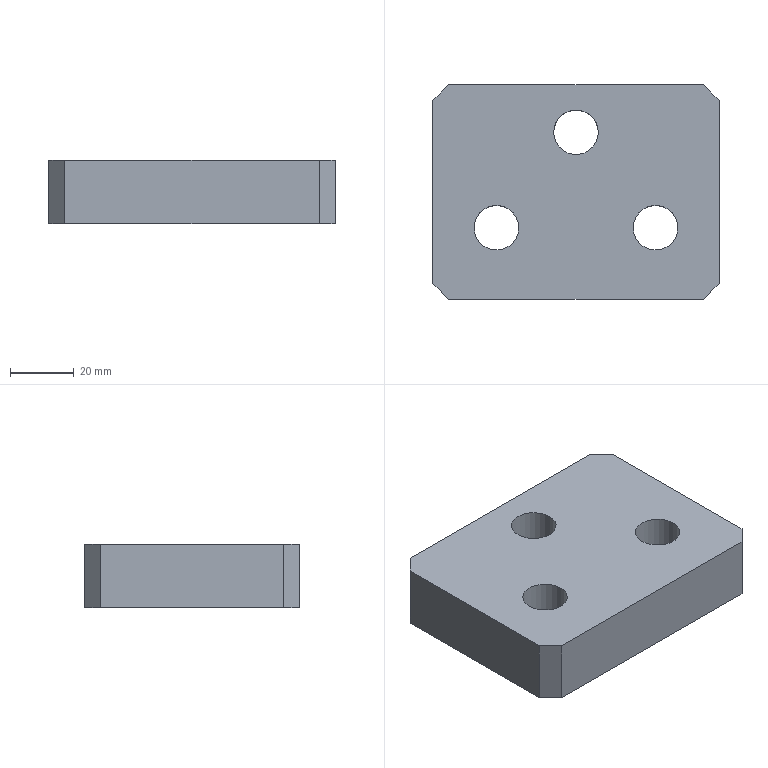Part | STEP file | 1_id1478_x_t | 1 solid | 13 faces | box 90 x 67.5 x 20 mm | volume 111264 mm3 | plane 10 | cylinder 3 | commonest cylinder face diameters 14 x3
STEP:
#1=CARTESIAN_POINT('',(0.,0.,0.));
#2=DIRECTION('',(0.,0.,1.));
#3=DIRECTION('',(1.,0.,0.));
#4=AXIS2_PLACEMENT_3D('',#1,#2,#3);
#5=CARTESIAN_POINT('',(837.95,375.5,-51.89));
#6=VERTEX_POINT('',#5);
#7=CARTESIAN_POINT('',(837.95,375.5,-71.89));
#8=VERTEX_POINT('',#7);
#9=CARTESIAN_POINT('',(837.95,375.5,-51.89));
#10=DIRECTION('',(0.,0.,-1.));
#11=VECTOR('',#10,1.);
#12=LINE('',#9,#11);
#13=CARTESIAN_POINT('',(832.95,375.5,-71.89));
#14=DIRECTION('',(0.,1.,0.));
#15=DIRECTION('',(-1.,0.,0.));
#16=AXIS2_PLACEMENT_3D('',#13,#14,#15);
#17=PLANE('',#16);
#18=CARTESIAN_POINT('',(-5.,20.));
#19=DIRECTION('',(0.,-1.));
#20=VECTOR('',#19,1.);
#21=LINE('',#18,#20);
#22=(GEOMETRIC_REPRESENTATION_CONTEXT(2)PARAMETRIC_REPRESENTATION_CONTEXT()REPRESENTATION_CONTEXT('',''));
#23=DEFINITIONAL_REPRESENTATION('',(#21),#22);
#24=PCURVE('',#17,#23);
#25=CARTESIAN_POINT('',(989.753,223.697,-71.89));
#26=DIRECTION('',(0.7071,0.7071,0.));
#27=DIRECTION('',(-0.7071,0.7071,0.));
#28=AXIS2_PLACEMENT_3D('',#25,#26,#27);
#29=PLANE('',#28);
#30=CARTESIAN_POINT('',(214.682,20.));
#31=DIRECTION('',(0.,-1.));
#32=VECTOR('',#31,1.);
#33=LINE('',#30,#32);
#34=(GEOMETRIC_REPRESENTATION_CONTEXT(2)PARAMETRIC_REPRESENTATION_CONTEXT()REPRESENTATION_CONTEXT('',''));
#35=DEFINITIONAL_REPRESENTATION('',(#33),#34);
#36=PCURVE('',#29,#35);
#37=SURFACE_CURVE('',#12,(#24,#36),.PCURVE_S1.);
#38=EDGE_CURVE('',#6,#8,#37,.T.);
#39=ORIENTED_EDGE('',*,*,#38,.T.);
#40=CARTESIAN_POINT('',(917.95,375.5,-71.89));
#41=VERTEX_POINT('',#40);
#42=CARTESIAN_POINT('',(917.95,375.5,-71.89));
#43=DIRECTION('',(-1.,0.,0.));
#44=VECTOR('',#43,1.);
#45=LINE('',#42,#44);
#46=CARTESIAN_POINT('',(-85.,0.));
#47=DIRECTION('',(1.,0.));
#48=VECTOR('',#47,1.);
#49=LINE('',#46,#48);
#50=(GEOMETRIC_REPRESENTATION_CONTEXT(2)PARAMETRIC_REPRESENTATION_CONTEXT()REPRESENTATION_CONTEXT('',''));
#51=DEFINITIONAL_REPRESENTATION('',(#49),#50);
#52=PCURVE('',#17,#51);
#53=CARTESIAN_POINT('',(739.556,-72.,-71.89));
#54=DIRECTION('',(0.,0.,1.));
#55=DIRECTION('',(1.,0.,0.));
#56=AXIS2_PLACEMENT_3D('',#53,#54,#55);
#57=PLANE('',#56);
#58=CARTESIAN_POINT('',(178.394,447.5));
#59=DIRECTION('',(-1.,0.));
#60=VECTOR('',#59,1.);
#61=LINE('',#58,#60);
#62=(GEOMETRIC_REPRESENTATION_CONTEXT(2)PARAMETRIC_REPRESENTATION_CONTEXT()REPRESENTATION_CONTEXT('',''));
#63=DEFINITIONAL_REPRESENTATION('',(#61),#62);
#64=PCURVE('',#57,#63);
#65=SURFACE_CURVE('',#45,(#52,#64),.PCURVE_S1.);
#66=EDGE_CURVE('',#41,#8,#65,.T.);
#67=ORIENTED_EDGE('',*,*,#66,.F.);
#68=CARTESIAN_POINT('',(917.95,375.5,-51.89));
#69=VERTEX_POINT('',#68);
#70=CARTESIAN_POINT('',(917.95,375.5,-51.89));
#71=DIRECTION('',(0.,0.,-1.));
#72=VECTOR('',#71,1.);
#73=LINE('',#70,#72);
#74=CARTESIAN_POINT('',(-85.,20.));
#75=DIRECTION('',(0.,-1.));
#76=VECTOR('',#75,1.);
#77=LINE('',#74,#76);
#78=(GEOMETRIC_REPRESENTATION_CONTEXT(2)PARAMETRIC_REPRESENTATION_CONTEXT()REPRESENTATION_CONTEXT('',''));
#79=DEFINITIONAL_REPRESENTATION('',(#77),#78);
#80=PCURVE('',#17,#79);
#81=CARTESIAN_POINT('',(577.753,35.303,-71.89));
#82=DIRECTION('',(-0.7071,0.7071,0.));
#83=DIRECTION('',(-0.7071,-0.7071,0.));
#84=AXIS2_PLACEMENT_3D('',#81,#82,#83);
#85=PLANE('',#84);
#86=CARTESIAN_POINT('',(-481.111,20.));
#87=DIRECTION('',(0.,-1.));
#88=VECTOR('',#87,1.);
#89=LINE('',#86,#88);
#90=(GEOMETRIC_REPRESENTATION_CONTEXT(2)PARAMETRIC_REPRESENTATION_CONTEXT()REPRESENTATION_CONTEXT('',''));
#91=DEFINITIONAL_REPRESENTATION('',(#89),#90);
#92=PCURVE('',#85,#91);
#93=SURFACE_CURVE('',#73,(#80,#92),.PCURVE_S1.);
#94=EDGE_CURVE('',#69,#41,#93,.T.);
#95=ORIENTED_EDGE('',*,*,#94,.F.);
#96=CARTESIAN_POINT('',(917.95,375.5,-51.89));
#97=DIRECTION('',(-1.,0.,0.));
#98=VECTOR('',#97,1.);
#99=LINE('',#96,#98);
#100=CARTESIAN_POINT('',(-85.,20.));
#101=DIRECTION('',(1.,0.));
#102=VECTOR('',#101,1.);
#103=LINE('',#100,#102);
#104=(GEOMETRIC_REPRESENTATION_CONTEXT(2)PARAMETRIC_REPRESENTATION_CONTEXT()REPRESENTATION_CONTEXT('',''));
#105=DEFINITIONAL_REPRESENTATION('',(#103),#104);
#106=PCURVE('',#17,#105);
#107=CARTESIAN_POINT('',(739.556,-72.,-51.89));
#108=DIRECTION('',(0.,0.,1.));
#109=DIRECTION('',(1.,0.,0.));
#110=AXIS2_PLACEMENT_3D('',#107,#108,#109);
#111=PLANE('',#110);
#112=CARTESIAN_POINT('',(178.394,447.5));
#113=DIRECTION('',(-1.,0.));
#114=VECTOR('',#113,1.);
#115=LINE('',#112,#114);
#116=(GEOMETRIC_REPRESENTATION_CONTEXT(2)PARAMETRIC_REPRESENTATION_CONTEXT()REPRESENTATION_CONTEXT('',''));
#117=DEFINITIONAL_REPRESENTATION('',(#115),#116);
#118=PCURVE('',#111,#117);
#119=SURFACE_CURVE('',#99,(#106,#118),.PCURVE_S1.);
#120=EDGE_CURVE('',#69,#6,#119,.T.);
#121=ORIENTED_EDGE('',*,*,#120,.T.);
#122=EDGE_LOOP('',(#39,#67,#95,#121));
#123=FACE_BOUND('',#122,.T.);
#124=ADVANCED_FACE('',(#123),#17,.F.);
#125=CARTESIAN_POINT('',(922.95,380.5,-51.89));
#126=VERTEX_POINT('',#125);
#127=CARTESIAN_POINT('',(917.95,375.5,-51.89));
#128=DIRECTION('',(0.7071,0.7071,0.));
#129=VECTOR('',#128,1.);
#130=LINE('',#127,#129);
#131=CARTESIAN_POINT('',(178.394,447.5));
#132=DIRECTION('',(0.7071,0.7071));
#133=VECTOR('',#132,1.);
#134=LINE('',#131,#133);
#135=(GEOMETRIC_REPRESENTATION_CONTEXT(2)PARAMETRIC_REPRESENTATION_CONTEXT()REPRESENTATION_CONTEXT('',''));
#136=DEFINITIONAL_REPRESENTATION('',(#134),#135);
#137=PCURVE('',#111,#136);
#138=CARTESIAN_POINT('',(-481.111,20.));
#139=DIRECTION('',(-1.,0.));
#140=VECTOR('',#139,1.);
#141=LINE('',#138,#140);
#142=(GEOMETRIC_REPRESENTATION_CONTEXT(2)PARAMETRIC_REPRESENTATION_CONTEXT()REPRESENTATION_CONTEXT('',''));
#143=DEFINITIONAL_REPRESENTATION('',(#141),#142);
#144=PCURVE('',#85,#143);
#145=SURFACE_CURVE('',#130,(#137,#144),.PCURVE_S1.);
#146=EDGE_CURVE('',#69,#126,#145,.T.);
#147=ORIENTED_EDGE('',*,*,#146,.T.);
#148=CARTESIAN_POINT('',(922.95,438.,-51.89));
#149=VERTEX_POINT('',#148);
#150=CARTESIAN_POINT('',(922.95,438.,-51.89));
#151=DIRECTION('',(0.,-1.,0.));
#152=VECTOR('',#151,1.);
#153=LINE('',#150,#152);
#154=CARTESIAN_POINT('',(183.394,510.));
#155=DIRECTION('',(0.,-1.));
#156=VECTOR('',#155,1.);
#157=LINE('',#154,#156);
#158=(GEOMETRIC_REPRESENTATION_CONTEXT(2)PARAMETRIC_REPRESENTATION_CONTEXT()REPRESENTATION_CONTEXT('',''));
#159=DEFINITIONAL_REPRESENTATION('',(#157),#158);
#160=PCURVE('',#111,#159);
#161=CARTESIAN_POINT('',(922.95,435.,-71.89));
#162=DIRECTION('',(-1.,0.,0.));
#163=DIRECTION('',(0.,-1.,0.));
#164=AXIS2_PLACEMENT_3D('',#161,#162,#163);
#165=PLANE('',#164);
#166=CARTESIAN_POINT('',(-3.,20.));
#167=DIRECTION('',(1.,0.));
#168=VECTOR('',#167,1.);
#169=LINE('',#166,#168);
#170=(GEOMETRIC_REPRESENTATION_CONTEXT(2)PARAMETRIC_REPRESENTATION_CONTEXT()REPRESENTATION_CONTEXT('',''));
#171=DEFINITIONAL_REPRESENTATION('',(#169),#170);
#172=PCURVE('',#165,#171);
#173=SURFACE_CURVE('',#153,(#160,#172),.PCURVE_S1.);
#174=EDGE_CURVE('',#149,#126,#173,.T.);
#175=ORIENTED_EDGE('',*,*,#174,.F.);
#176=CARTESIAN_POINT('',(917.95,443.,-51.89));
#177=VERTEX_POINT('',#176);
#178=CARTESIAN_POINT('',(922.95,438.,-51.89));
#179=DIRECTION('',(-0.7071,0.7071,0.));
#180=VECTOR('',#179,1.);
#181=LINE('',#178,#180);
#182=CARTESIAN_POINT('',(183.394,510.));
#183=DIRECTION('',(-0.7071,0.7071));
#184=VECTOR('',#183,1.);
#185=LINE('',#182,#184);
#186=(GEOMETRIC_REPRESENTATION_CONTEXT(2)PARAMETRIC_REPRESENTATION_CONTEXT()REPRESENTATION_CONTEXT('',''));
#187=DEFINITIONAL_REPRESENTATION('',(#185),#186);
#188=PCURVE('',#111,#187);
#189=CARTESIAN_POINT('',(1061.253,299.697,-71.89));
#190=DIRECTION('',(-0.7071,-0.7071,0.));
#191=DIRECTION('',(0.7071,-0.7071,0.));
#192=AXIS2_PLACEMENT_3D('',#189,#190,#191);
#193=PLANE('',#192);
#194=CARTESIAN_POINT('',(-195.59,20.));
#195=DIRECTION('',(-1.,0.));
#196=VECTOR('',#195,1.);
#197=LINE('',#194,#196);
#198=(GEOMETRIC_REPRESENTATION_CONTEXT(2)PARAMETRIC_REPRESENTATION_CONTEXT()REPRESENTATION_CONTEXT('',''));
#199=DEFINITIONAL_REPRESENTATION('',(#197),#198);
#200=PCURVE('',#193,#199);
#201=SURFACE_CURVE('',#181,(#188,#200),.PCURVE_S1.);
#202=EDGE_CURVE('',#149,#177,#201,.T.);
#203=ORIENTED_EDGE('',*,*,#202,.T.);
#204=CARTESIAN_POINT('',(837.95,443.,-51.89));
#205=VERTEX_POINT('',#204);
#206=CARTESIAN_POINT('',(837.95,443.,-51.89));
#207=DIRECTION('',(1.,0.,0.));
#208=VECTOR('',#207,1.);
#209=LINE('',#206,#208);
#210=CARTESIAN_POINT('',(98.394,515.));
#211=DIRECTION('',(1.,0.));
#212=VECTOR('',#211,1.);
#213=LINE('',#210,#212);
#214=(GEOMETRIC_REPRESENTATION_CONTEXT(2)PARAMETRIC_REPRESENTATION_CONTEXT()REPRESENTATION_CONTEXT('',''));
#215=DEFINITIONAL_REPRESENTATION('',(#213),#214);
#216=PCURVE('',#111,#215);
#217=CARTESIAN_POINT('',(834.95,443.,-71.89));
#218=DIRECTION('',(0.,-1.,0.));
#219=DIRECTION('',(1.,0.,0.));
#220=AXIS2_PLACEMENT_3D('',#217,#218,#219);
#221=PLANE('',#220);
#222=CARTESIAN_POINT('',(3.,20.));
#223=DIRECTION('',(1.,0.));
#224=VECTOR('',#223,1.);
#225=LINE('',#222,#224);
#226=(GEOMETRIC_REPRESENTATION_CONTEXT(2)PARAMETRIC_REPRESENTATION_CONTEXT()REPRESENTATION_CONTEXT('',''));
#227=DEFINITIONAL_REPRESENTATION('',(#225),#226);
#228=PCURVE('',#221,#227);
#229=SURFACE_CURVE('',#209,(#216,#228),.PCURVE_S1.);
#230=EDGE_CURVE('',#205,#177,#229,.T.);
#231=ORIENTED_EDGE('',*,*,#230,.F.);
#232=CARTESIAN_POINT('',(832.95,438.,-51.89));
#233=VERTEX_POINT('',#232);
#234=CARTESIAN_POINT('',(837.95,443.,-51.89));
#235=DIRECTION('',(-0.7071,-0.7071,0.));
#236=VECTOR('',#235,1.);
#237=LINE('',#234,#236);
#238=CARTESIAN_POINT('',(98.394,515.));
#239=DIRECTION('',(-0.7071,-0.7071));
#240=VECTOR('',#239,1.);
#241=LINE('',#238,#240);
#242=(GEOMETRIC_REPRESENTATION_CONTEXT(2)PARAMETRIC_REPRESENTATION_CONTEXT()REPRESENTATION_CONTEXT('',''));
#243=DEFINITIONAL_REPRESENTATION('',(#241),#242);
#244=PCURVE('',#111,#243);
#245=CARTESIAN_POINT('',(506.253,111.303,-71.89));
#246=DIRECTION('',(0.7071,-0.7071,0.));
#247=DIRECTION('',(0.7071,0.7071,0.));
#248=AXIS2_PLACEMENT_3D('',#245,#246,#247);
#249=PLANE('',#248);
#250=CARTESIAN_POINT('',(469.091,20.));
#251=DIRECTION('',(-1.,0.));
#252=VECTOR('',#251,1.);
#253=LINE('',#250,#252);
#254=(GEOMETRIC_REPRESENTATION_CONTEXT(2)PARAMETRIC_REPRESENTATION_CONTEXT()REPRESENTATION_CONTEXT('',''));
#255=DEFINITIONAL_REPRESENTATION('',(#253),#254);
#256=PCURVE('',#249,#255);
#257=SURFACE_CURVE('',#237,(#244,#256),.PCURVE_S1.);
#258=EDGE_CURVE('',#205,#233,#257,.T.);
#259=ORIENTED_EDGE('',*,*,#258,.T.);
#260=CARTESIAN_POINT('',(832.95,380.5,-51.89));
#261=VERTEX_POINT('',#260);
#262=CARTESIAN_POINT('',(832.95,380.5,-51.89));
#263=DIRECTION('',(0.,1.,0.));
#264=VECTOR('',#263,1.);
#265=LINE('',#262,#264);
#266=CARTESIAN_POINT('',(93.394,452.5));
#267=DIRECTION('',(0.,1.));
#268=VECTOR('',#267,1.);
#269=LINE('',#266,#268);
#270=(GEOMETRIC_REPRESENTATION_CONTEXT(2)PARAMETRIC_REPRESENTATION_CONTEXT()REPRESENTATION_CONTEXT('',''));
#271=DEFINITIONAL_REPRESENTATION('',(#269),#270);
#272=PCURVE('',#111,#271);
#273=CARTESIAN_POINT('',(832.95,364.,-71.89));
#274=DIRECTION('',(1.,0.,0.));
#275=DIRECTION('',(0.,1.,0.));
#276=AXIS2_PLACEMENT_3D('',#273,#274,#275);
#277=PLANE('',#276);
#278=CARTESIAN_POINT('',(16.5,20.));
#279=DIRECTION('',(1.,0.));
#280=VECTOR('',#279,1.);
#281=LINE('',#278,#280);
#282=(GEOMETRIC_REPRESENTATION_CONTEXT(2)PARAMETRIC_REPRESENTATION_CONTEXT()REPRESENTATION_CONTEXT('',''));
#283=DEFINITIONAL_REPRESENTATION('',(#281),#282);
#284=PCURVE('',#277,#283);
#285=SURFACE_CURVE('',#265,(#272,#284),.PCURVE_S1.);
#286=EDGE_CURVE('',#261,#233,#285,.T.);
#287=ORIENTED_EDGE('',*,*,#286,.F.);
#288=CARTESIAN_POINT('',(832.95,380.5,-51.89));
#289=DIRECTION('',(0.7071,-0.7071,0.));
#290=VECTOR('',#289,1.);
#291=LINE('',#288,#290);
#292=CARTESIAN_POINT('',(93.394,452.5));
#293=DIRECTION('',(0.7071,-0.7071));
#294=VECTOR('',#293,1.);
#295=LINE('',#292,#294);
#296=(GEOMETRIC_REPRESENTATION_CONTEXT(2)PARAMETRIC_REPRESENTATION_CONTEXT()REPRESENTATION_CONTEXT('',''));
#297=DEFINITIONAL_REPRESENTATION('',(#295),#296);
#298=PCURVE('',#111,#297);
#299=CARTESIAN_POINT('',(221.753,20.));
#300=DIRECTION('',(-1.,0.));
#301=VECTOR('',#300,1.);
#302=LINE('',#299,#301);
#303=(GEOMETRIC_REPRESENTATION_CONTEXT(2)PARAMETRIC_REPRESENTATION_CONTEXT()REPRESENTATION_CONTEXT('',''));
#304=DEFINITIONAL_REPRESENTATION('',(#302),#303);
#305=PCURVE('',#29,#304);
#306=SURFACE_CURVE('',#291,(#298,#305),.PCURVE_S1.);
#307=EDGE_CURVE('',#261,#6,#306,.T.);
#308=ORIENTED_EDGE('',*,*,#307,.T.);
#309=ORIENTED_EDGE('',*,*,#120,.F.);
#310=EDGE_LOOP('',(#147,#175,#203,#231,#259,#287,#308,#309));
#311=FACE_BOUND('',#310,.T.);
#312=CARTESIAN_POINT('',(895.95,398.,-51.89));
#313=VERTEX_POINT('',#312);
#314=CARTESIAN_POINT('',(902.95,398.,-51.89));
#315=DIRECTION('',(0.,0.,-1.));
#316=DIRECTION('',(-1.,0.,0.));
#317=AXIS2_PLACEMENT_3D('',#314,#315,#316);
#318=CIRCLE('',#317,7.);
#319=CARTESIAN_POINT('',(156.394,470.));
#320=CARTESIAN_POINT('',(156.394,482.124));
#321=CARTESIAN_POINT('',(166.894,476.062));
#322=CARTESIAN_POINT('',(177.394,470.));
#323=CARTESIAN_POINT('',(166.894,463.938));
#324=CARTESIAN_POINT('',(156.394,457.876));
#325=CARTESIAN_POINT('',(156.394,470.));
#326=(BOUNDED_CURVE()B_SPLINE_CURVE(2,(#319,#320,#321,#322,#323,#324,#325),.UNSPECIFIED.,.T.,.F.)B_SPLINE_CURVE_WITH_KNOTS((1,2,2,2,2,1),(-2.094,0.,2.094,4.189,6.283,8.378),.UNSPECIFIED.)CURVE()GEOMETRIC_REPRESENTATION_ITEM()RATIONAL_B_SPLINE_CURVE((1.,0.5,1.,0.5,1.,0.5,1.))REPRESENTATION_ITEM(''));
#327=(GEOMETRIC_REPRESENTATION_CONTEXT(2)PARAMETRIC_REPRESENTATION_CONTEXT()REPRESENTATION_CONTEXT('',''));
#328=DEFINITIONAL_REPRESENTATION('',(#326),#327);
#329=PCURVE('',#111,#328);
#330=CARTESIAN_POINT('',(902.95,398.,-71.89));
#331=DIRECTION('',(0.,0.,1.));
#332=DIRECTION('',(-1.,0.,0.));
#333=AXIS2_PLACEMENT_3D('',#330,#331,#332);
#334=CYLINDRICAL_SURFACE('',#333,7.);
#335=CARTESIAN_POINT('',(6.283,20.));
#336=DIRECTION('',(-1.,0.));
#337=VECTOR('',#336,1.);
#338=LINE('',#335,#337);
#339=(GEOMETRIC_REPRESENTATION_CONTEXT(2)PARAMETRIC_REPRESENTATION_CONTEXT()REPRESENTATION_CONTEXT('',''));
#340=DEFINITIONAL_REPRESENTATION('',(#338),#339);
#341=PCURVE('',#334,#340);
#342=SURFACE_CURVE('',#318,(#329,#341),.PCURVE_S1.);
#343=EDGE_CURVE('',#313,#313,#342,.T.);
#344=ORIENTED_EDGE('',*,*,#343,.T.);
#345=EDGE_LOOP('',(#344));
#346=FACE_BOUND('',#345,.T.);
#347=CARTESIAN_POINT('',(845.95,398.,-51.89));
#348=VERTEX_POINT('',#347);
#349=CARTESIAN_POINT('',(852.95,398.,-51.89));
#350=DIRECTION('',(0.,0.,-1.));
#351=DIRECTION('',(-1.,0.,0.));
#352=AXIS2_PLACEMENT_3D('',#349,#350,#351);
#353=CIRCLE('',#352,7.);
#354=CARTESIAN_POINT('',(106.394,470.));
#355=CARTESIAN_POINT('',(106.394,482.124));
#356=CARTESIAN_POINT('',(116.894,476.062));
#357=CARTESIAN_POINT('',(127.394,470.));
#358=CARTESIAN_POINT('',(116.894,463.938));
#359=CARTESIAN_POINT('',(106.394,457.876));
#360=CARTESIAN_POINT('',(106.394,470.));
#361=(BOUNDED_CURVE()B_SPLINE_CURVE(2,(#354,#355,#356,#357,#358,#359,#360),.UNSPECIFIED.,.T.,.F.)B_SPLINE_CURVE_WITH_KNOTS((1,2,2,2,2,1),(-2.094,0.,2.094,4.189,6.283,8.378),.UNSPECIFIED.)CURVE()GEOMETRIC_REPRESENTATION_ITEM()RATIONAL_B_SPLINE_CURVE((1.,0.5,1.,0.5,1.,0.5,1.))REPRESENTATION_ITEM(''));
#362=(GEOMETRIC_REPRESENTATION_CONTEXT(2)PARAMETRIC_REPRESENTATION_CONTEXT()REPRESENTATION_CONTEXT('',''));
#363=DEFINITIONAL_REPRESENTATION('',(#361),#362);
#364=PCURVE('',#111,#363);
#365=CARTESIAN_POINT('',(852.95,398.,-71.89));
#366=DIRECTION('',(0.,0.,1.));
#367=DIRECTION('',(-1.,0.,0.));
#368=AXIS2_PLACEMENT_3D('',#365,#366,#367);
#369=CYLINDRICAL_SURFACE('',#368,7.);
#370=CARTESIAN_POINT('',(6.283,20.));
#371=DIRECTION('',(-1.,0.));
#372=VECTOR('',#371,1.);
#373=LINE('',#370,#372);
#374=(GEOMETRIC_REPRESENTATION_CONTEXT(2)PARAMETRIC_REPRESENTATION_CONTEXT()REPRESENTATION_CONTEXT('',''));
#375=DEFINITIONAL_REPRESENTATION('',(#373),#374);
#376=PCURVE('',#369,#375);
#377=SURFACE_CURVE('',#353,(#364,#376),.PCURVE_S1.);
#378=EDGE_CURVE('',#348,#348,#377,.T.);
#379=ORIENTED_EDGE('',*,*,#378,.T.);
#380=EDGE_LOOP('',(#379));
#381=FACE_BOUND('',#380,.T.);
#382=CARTESIAN_POINT('',(870.95,428.,-51.89));
#383=VERTEX_POINT('',#382);
#384=CARTESIAN_POINT('',(877.95,428.,-51.89));
#385=DIRECTION('',(0.,0.,-1.));
#386=DIRECTION('',(-1.,0.,0.));
#387=AXIS2_PLACEMENT_3D('',#384,#385,#386);
#388=CIRCLE('',#387,7.);
#389=CARTESIAN_POINT('',(131.394,500.));
#390=CARTESIAN_POINT('',(131.394,512.124));
#391=CARTESIAN_POINT('',(141.894,506.062));
#392=CARTESIAN_POINT('',(152.394,500.));
#393=CARTESIAN_POINT('',(141.894,493.938));
#394=CARTESIAN_POINT('',(131.394,487.876));
#395=CARTESIAN_POINT('',(131.394,500.));
#396=(BOUNDED_CURVE()B_SPLINE_CURVE(2,(#389,#390,#391,#392,#393,#394,#395),.UNSPECIFIED.,.T.,.F.)B_SPLINE_CURVE_WITH_KNOTS((1,2,2,2,2,1),(-2.094,0.,2.094,4.189,6.283,8.378),.UNSPECIFIED.)CURVE()GEOMETRIC_REPRESENTATION_ITEM()RATIONAL_B_SPLINE_CURVE((1.,0.5,1.,0.5,1.,0.5,1.))REPRESENTATION_ITEM(''));
#397=(GEOMETRIC_REPRESENTATION_CONTEXT(2)PARAMETRIC_REPRESENTATION_CONTEXT()REPRESENTATION_CONTEXT('',''));
#398=DEFINITIONAL_REPRESENTATION('',(#396),#397);
#399=PCURVE('',#111,#398);
#400=CARTESIAN_POINT('',(877.95,428.,-71.89));
#401=DIRECTION('',(0.,0.,1.));
#402=DIRECTION('',(-1.,0.,0.));
#403=AXIS2_PLACEMENT_3D('',#400,#401,#402);
#404=CYLINDRICAL_SURFACE('',#403,7.);
#405=CARTESIAN_POINT('',(6.283,20.));
#406=DIRECTION('',(-1.,0.));
#407=VECTOR('',#406,1.);
#408=LINE('',#405,#407);
#409=(GEOMETRIC_REPRESENTATION_CONTEXT(2)PARAMETRIC_REPRESENTATION_CONTEXT()REPRESENTATION_CONTEXT('',''));
#410=DEFINITIONAL_REPRESENTATION('',(#408),#409);
#411=PCURVE('',#404,#410);
#412=SURFACE_CURVE('',#388,(#399,#411),.PCURVE_S1.);
#413=EDGE_CURVE('',#383,#383,#412,.T.);
#414=ORIENTED_EDGE('',*,*,#413,.T.);
#415=EDGE_LOOP('',(#414));
#416=FACE_BOUND('',#415,.T.);
#417=ADVANCED_FACE('',(#311,#346,#381,#416),#111,.T.);
#418=CARTESIAN_POINT('',(832.95,380.5,-71.89));
#419=VERTEX_POINT('',#418);
#420=CARTESIAN_POINT('',(832.95,380.5,-51.89));
#421=DIRECTION('',(0.,0.,-1.));
#422=VECTOR('',#421,1.);
#423=LINE('',#420,#422);
#424=CARTESIAN_POINT('',(221.753,20.));
#425=DIRECTION('',(0.,-1.));
#426=VECTOR('',#425,1.);
#427=LINE('',#424,#426);
#428=(GEOMETRIC_REPRESENTATION_CONTEXT(2)PARAMETRIC_REPRESENTATION_CONTEXT()REPRESENTATION_CONTEXT('',''));
#429=DEFINITIONAL_REPRESENTATION('',(#427),#428);
#430=PCURVE('',#29,#429);
#431=CARTESIAN_POINT('',(16.5,20.));
#432=DIRECTION('',(0.,-1.));
#433=VECTOR('',#432,1.);
#434=LINE('',#431,#433);
#435=(GEOMETRIC_REPRESENTATION_CONTEXT(2)PARAMETRIC_REPRESENTATION_CONTEXT()REPRESENTATION_CONTEXT('',''));
#436=DEFINITIONAL_REPRESENTATION('',(#434),#435);
#437=PCURVE('',#277,#436);
#438=SURFACE_CURVE('',#423,(#430,#437),.PCURVE_S1.);
#439=EDGE_CURVE('',#261,#419,#438,.T.);
#440=ORIENTED_EDGE('',*,*,#439,.T.);
#441=CARTESIAN_POINT('',(837.95,375.5,-71.89));
#442=DIRECTION('',(-0.7071,0.7071,0.));
#443=VECTOR('',#442,1.);
#444=LINE('',#441,#443);
#445=CARTESIAN_POINT('',(214.682,0.));
#446=DIRECTION('',(1.,0.));
#447=VECTOR('',#446,1.);
#448=LINE('',#445,#447);
#449=(GEOMETRIC_REPRESENTATION_CONTEXT(2)PARAMETRIC_REPRESENTATION_CONTEXT()REPRESENTATION_CONTEXT('',''));
#450=DEFINITIONAL_REPRESENTATION('',(#448),#449);
#451=PCURVE('',#29,#450);
#452=CARTESIAN_POINT('',(98.394,447.5));
#453=DIRECTION('',(-0.7071,0.7071));
#454=VECTOR('',#453,1.);
#455=LINE('',#452,#454);
#456=(GEOMETRIC_REPRESENTATION_CONTEXT(2)PARAMETRIC_REPRESENTATION_CONTEXT()REPRESENTATION_CONTEXT('',''));
#457=DEFINITIONAL_REPRESENTATION('',(#455),#456);
#458=PCURVE('',#57,#457);
#459=SURFACE_CURVE('',#444,(#451,#458),.PCURVE_S1.);
#460=EDGE_CURVE('',#8,#419,#459,.T.);
#461=ORIENTED_EDGE('',*,*,#460,.F.);
#462=ORIENTED_EDGE('',*,*,#38,.F.);
#463=ORIENTED_EDGE('',*,*,#307,.F.);
#464=EDGE_LOOP('',(#440,#461,#462,#463));
#465=FACE_BOUND('',#464,.T.);
#466=ADVANCED_FACE('',(#465),#29,.F.);
#467=ORIENTED_EDGE('',*,*,#460,.T.);
#468=CARTESIAN_POINT('',(832.95,438.,-71.89));
#469=VERTEX_POINT('',#468);
#470=CARTESIAN_POINT('',(832.95,380.5,-71.89));
#471=DIRECTION('',(0.,1.,0.));
#472=VECTOR('',#471,1.);
#473=LINE('',#470,#472);
#474=CARTESIAN_POINT('',(93.394,452.5));
#475=DIRECTION('',(0.,1.));
#476=VECTOR('',#475,1.);
#477=LINE('',#474,#476);
#478=(GEOMETRIC_REPRESENTATION_CONTEXT(2)PARAMETRIC_REPRESENTATION_CONTEXT()REPRESENTATION_CONTEXT('',''));
#479=DEFINITIONAL_REPRESENTATION('',(#477),#478);
#480=PCURVE('',#57,#479);
#481=CARTESIAN_POINT('',(16.5,0.));
#482=DIRECTION('',(1.,0.));
#483=VECTOR('',#482,1.);
#484=LINE('',#481,#483);
#485=(GEOMETRIC_REPRESENTATION_CONTEXT(2)PARAMETRIC_REPRESENTATION_CONTEXT()REPRESENTATION_CONTEXT('',''));
#486=DEFINITIONAL_REPRESENTATION('',(#484),#485);
#487=PCURVE('',#277,#486);
#488=SURFACE_CURVE('',#473,(#480,#487),.PCURVE_S1.);
#489=EDGE_CURVE('',#419,#469,#488,.T.);
#490=ORIENTED_EDGE('',*,*,#489,.T.);
#491=CARTESIAN_POINT('',(837.95,443.,-71.89));
#492=VERTEX_POINT('',#491);
#493=CARTESIAN_POINT('',(832.95,438.,-71.89));
#494=DIRECTION('',(0.7071,0.7071,0.));
#495=VECTOR('',#494,1.);
#496=LINE('',#493,#495);
#497=CARTESIAN_POINT('',(93.394,510.));
#498=DIRECTION('',(0.7071,0.7071));
#499=VECTOR('',#498,1.);
#500=LINE('',#497,#499);
#501=(GEOMETRIC_REPRESENTATION_CONTEXT(2)PARAMETRIC_REPRESENTATION_CONTEXT()REPRESENTATION_CONTEXT('',''));
#502=DEFINITIONAL_REPRESENTATION('',(#500),#501);
#503=PCURVE('',#57,#502);
#504=CARTESIAN_POINT('',(462.019,0.));
#505=DIRECTION('',(1.,0.));
#506=VECTOR('',#505,1.);
#507=LINE('',#504,#506);
#508=(GEOMETRIC_REPRESENTATION_CONTEXT(2)PARAMETRIC_REPRESENTATION_CONTEXT()REPRESENTATION_CONTEXT('',''));
#509=DEFINITIONAL_REPRESENTATION('',(#507),#508);
#510=PCURVE('',#249,#509);
#511=SURFACE_CURVE('',#496,(#503,#510),.PCURVE_S1.);
#512=EDGE_CURVE('',#469,#492,#511,.T.);
#513=ORIENTED_EDGE('',*,*,#512,.T.);
#514=CARTESIAN_POINT('',(917.95,443.,-71.89));
#515=VERTEX_POINT('',#514);
#516=CARTESIAN_POINT('',(837.95,443.,-71.89));
#517=DIRECTION('',(1.,0.,0.));
#518=VECTOR('',#517,1.);
#519=LINE('',#516,#518);
#520=CARTESIAN_POINT('',(98.394,515.));
#521=DIRECTION('',(1.,0.));
#522=VECTOR('',#521,1.);
#523=LINE('',#520,#522);
#524=(GEOMETRIC_REPRESENTATION_CONTEXT(2)PARAMETRIC_REPRESENTATION_CONTEXT()REPRESENTATION_CONTEXT('',''));
#525=DEFINITIONAL_REPRESENTATION('',(#523),#524);
#526=PCURVE('',#57,#525);
#527=CARTESIAN_POINT('',(3.,0.));
#528=DIRECTION('',(1.,0.));
#529=VECTOR('',#528,1.);
#530=LINE('',#527,#529);
#531=(GEOMETRIC_REPRESENTATION_CONTEXT(2)PARAMETRIC_REPRESENTATION_CONTEXT()REPRESENTATION_CONTEXT('',''));
#532=DEFINITIONAL_REPRESENTATION('',(#530),#531);
#533=PCURVE('',#221,#532);
#534=SURFACE_CURVE('',#519,(#526,#533),.PCURVE_S1.);
#535=EDGE_CURVE('',#492,#515,#534,.T.);
#536=ORIENTED_EDGE('',*,*,#535,.T.);
#537=CARTESIAN_POINT('',(922.95,438.,-71.89));
#538=VERTEX_POINT('',#537);
#539=CARTESIAN_POINT('',(917.95,443.,-71.89));
#540=DIRECTION('',(0.7071,-0.7071,0.));
#541=VECTOR('',#540,1.);
#542=LINE('',#539,#541);
#543=CARTESIAN_POINT('',(178.394,515.));
#544=DIRECTION('',(0.7071,-0.7071));
#545=VECTOR('',#544,1.);
#546=LINE('',#543,#545);
#547=(GEOMETRIC_REPRESENTATION_CONTEXT(2)PARAMETRIC_REPRESENTATION_CONTEXT()REPRESENTATION_CONTEXT('',''));
#548=DEFINITIONAL_REPRESENTATION('',(#546),#547);
#549=PCURVE('',#57,#548);
#550=CARTESIAN_POINT('',(-202.661,0.));
#551=DIRECTION('',(1.,0.));
#552=VECTOR('',#551,1.);
#553=LINE('',#550,#552);
#554=(GEOMETRIC_REPRESENTATION_CONTEXT(2)PARAMETRIC_REPRESENTATION_CONTEXT()REPRESENTATION_CONTEXT('',''));
#555=DEFINITIONAL_REPRESENTATION('',(#553),#554);
#556=PCURVE('',#193,#555);
#557=SURFACE_CURVE('',#542,(#549,#556),.PCURVE_S1.);
#558=EDGE_CURVE('',#515,#538,#557,.T.);
#559=ORIENTED_EDGE('',*,*,#558,.T.);
#560=CARTESIAN_POINT('',(922.95,380.5,-71.89));
#561=VERTEX_POINT('',#560);
#562=CARTESIAN_POINT('',(922.95,438.,-71.89));
#563=DIRECTION('',(0.,-1.,0.));
#564=VECTOR('',#563,1.);
#565=LINE('',#562,#564);
#566=CARTESIAN_POINT('',(183.394,510.));
#567=DIRECTION('',(0.,-1.));
#568=VECTOR('',#567,1.);
#569=LINE('',#566,#568);
#570=(GEOMETRIC_REPRESENTATION_CONTEXT(2)PARAMETRIC_REPRESENTATION_CONTEXT()REPRESENTATION_CONTEXT('',''));
#571=DEFINITIONAL_REPRESENTATION('',(#569),#570);
#572=PCURVE('',#57,#571);
#573=CARTESIAN_POINT('',(-3.,0.));
#574=DIRECTION('',(1.,0.));
#575=VECTOR('',#574,1.);
#576=LINE('',#573,#575);
#577=(GEOMETRIC_REPRESENTATION_CONTEXT(2)PARAMETRIC_REPRESENTATION_CONTEXT()REPRESENTATION_CONTEXT('',''));
#578=DEFINITIONAL_REPRESENTATION('',(#576),#577);
#579=PCURVE('',#165,#578);
#580=SURFACE_CURVE('',#565,(#572,#579),.PCURVE_S1.);
#581=EDGE_CURVE('',#538,#561,#580,.T.);
#582=ORIENTED_EDGE('',*,*,#581,.T.);
#583=CARTESIAN_POINT('',(922.95,380.5,-71.89));
#584=DIRECTION('',(-0.7071,-0.7071,0.));
#585=VECTOR('',#584,1.);
#586=LINE('',#583,#585);
#587=CARTESIAN_POINT('',(183.394,452.5));
#588=DIRECTION('',(-0.7071,-0.7071));
#589=VECTOR('',#588,1.);
#590=LINE('',#587,#589);
#591=(GEOMETRIC_REPRESENTATION_CONTEXT(2)PARAMETRIC_REPRESENTATION_CONTEXT()REPRESENTATION_CONTEXT('',''));
#592=DEFINITIONAL_REPRESENTATION('',(#590),#591);
#593=PCURVE('',#57,#592);
#594=CARTESIAN_POINT('',(-488.182,0.));
#595=DIRECTION('',(1.,0.));
#596=VECTOR('',#595,1.);
#597=LINE('',#594,#596);
#598=(GEOMETRIC_REPRESENTATION_CONTEXT(2)PARAMETRIC_REPRESENTATION_CONTEXT()REPRESENTATION_CONTEXT('',''));
#599=DEFINITIONAL_REPRESENTATION('',(#597),#598);
#600=PCURVE('',#85,#599);
#601=SURFACE_CURVE('',#586,(#593,#600),.PCURVE_S1.);
#602=EDGE_CURVE('',#561,#41,#601,.T.);
#603=ORIENTED_EDGE('',*,*,#602,.T.);
#604=ORIENTED_EDGE('',*,*,#66,.T.);
#605=EDGE_LOOP('',(#467,#490,#513,#536,#559,#582,#603,#604));
#606=FACE_BOUND('',#605,.T.);
#607=CARTESIAN_POINT('',(895.95,398.,-71.89));
#608=VERTEX_POINT('',#607);
#609=CARTESIAN_POINT('',(902.95,398.,-71.89));
#610=DIRECTION('',(0.,0.,1.));
#611=DIRECTION('',(-1.,0.,0.));
#612=AXIS2_PLACEMENT_3D('',#609,#610,#611);
#613=CIRCLE('',#612,7.);
#614=CARTESIAN_POINT('',(163.394,470.));
#615=DIRECTION('',(-1.,0.));
#616=AXIS2_PLACEMENT_2D('',#614,#615);
#617=CIRCLE('',#616,7.);
#618=(GEOMETRIC_REPRESENTATION_CONTEXT(2)PARAMETRIC_REPRESENTATION_CONTEXT()REPRESENTATION_CONTEXT('',''));
#619=DEFINITIONAL_REPRESENTATION('',(#617),#618);
#620=PCURVE('',#57,#619);
#621=CARTESIAN_POINT('',(0.,0.));
#622=DIRECTION('',(1.,0.));
#623=VECTOR('',#622,1.);
#624=LINE('',#621,#623);
#625=(GEOMETRIC_REPRESENTATION_CONTEXT(2)PARAMETRIC_REPRESENTATION_CONTEXT()REPRESENTATION_CONTEXT('',''));
#626=DEFINITIONAL_REPRESENTATION('',(#624),#625);
#627=PCURVE('',#334,#626);
#628=SURFACE_CURVE('',#613,(#620,#627),.PCURVE_S1.);
#629=EDGE_CURVE('',#608,#608,#628,.T.);
#630=ORIENTED_EDGE('',*,*,#629,.T.);
#631=EDGE_LOOP('',(#630));
#632=FACE_BOUND('',#631,.T.);
#633=CARTESIAN_POINT('',(845.95,398.,-71.89));
#634=VERTEX_POINT('',#633);
#635=CARTESIAN_POINT('',(852.95,398.,-71.89));
#636=DIRECTION('',(0.,0.,1.));
#637=DIRECTION('',(-1.,0.,0.));
#638=AXIS2_PLACEMENT_3D('',#635,#636,#637);
#639=CIRCLE('',#638,7.);
#640=CARTESIAN_POINT('',(113.394,470.));
#641=DIRECTION('',(-1.,0.));
#642=AXIS2_PLACEMENT_2D('',#640,#641);
#643=CIRCLE('',#642,7.);
#644=(GEOMETRIC_REPRESENTATION_CONTEXT(2)PARAMETRIC_REPRESENTATION_CONTEXT()REPRESENTATION_CONTEXT('',''));
#645=DEFINITIONAL_REPRESENTATION('',(#643),#644);
#646=PCURVE('',#57,#645);
#647=CARTESIAN_POINT('',(0.,0.));
#648=DIRECTION('',(1.,0.));
#649=VECTOR('',#648,1.);
#650=LINE('',#647,#649);
#651=(GEOMETRIC_REPRESENTATION_CONTEXT(2)PARAMETRIC_REPRESENTATION_CONTEXT()REPRESENTATION_CONTEXT('',''));
#652=DEFINITIONAL_REPRESENTATION('',(#650),#651);
#653=PCURVE('',#369,#652);
#654=SURFACE_CURVE('',#639,(#646,#653),.PCURVE_S1.);
#655=EDGE_CURVE('',#634,#634,#654,.T.);
#656=ORIENTED_EDGE('',*,*,#655,.T.);
#657=EDGE_LOOP('',(#656));
#658=FACE_BOUND('',#657,.T.);
#659=CARTESIAN_POINT('',(870.95,428.,-71.89));
#660=VERTEX_POINT('',#659);
#661=CARTESIAN_POINT('',(877.95,428.,-71.89));
#662=DIRECTION('',(0.,0.,1.));
#663=DIRECTION('',(-1.,0.,0.));
#664=AXIS2_PLACEMENT_3D('',#661,#662,#663);
#665=CIRCLE('',#664,7.);
#666=CARTESIAN_POINT('',(138.394,500.));
#667=DIRECTION('',(-1.,0.));
#668=AXIS2_PLACEMENT_2D('',#666,#667);
#669=CIRCLE('',#668,7.);
#670=(GEOMETRIC_REPRESENTATION_CONTEXT(2)PARAMETRIC_REPRESENTATION_CONTEXT()REPRESENTATION_CONTEXT('',''));
#671=DEFINITIONAL_REPRESENTATION('',(#669),#670);
#672=PCURVE('',#57,#671);
#673=CARTESIAN_POINT('',(0.,0.));
#674=DIRECTION('',(1.,0.));
#675=VECTOR('',#674,1.);
#676=LINE('',#673,#675);
#677=(GEOMETRIC_REPRESENTATION_CONTEXT(2)PARAMETRIC_REPRESENTATION_CONTEXT()REPRESENTATION_CONTEXT('',''));
#678=DEFINITIONAL_REPRESENTATION('',(#676),#677);
#679=PCURVE('',#404,#678);
#680=SURFACE_CURVE('',#665,(#672,#679),.PCURVE_S1.);
#681=EDGE_CURVE('',#660,#660,#680,.T.);
#682=ORIENTED_EDGE('',*,*,#681,.T.);
#683=EDGE_LOOP('',(#682));
#684=FACE_BOUND('',#683,.T.);
#685=ADVANCED_FACE('',(#606,#632,#658,#684),#57,.F.);
#686=ORIENTED_EDGE('',*,*,#94,.T.);
#687=ORIENTED_EDGE('',*,*,#602,.F.);
#688=CARTESIAN_POINT('',(922.95,380.5,-51.89));
#689=DIRECTION('',(0.,0.,-1.));
#690=VECTOR('',#689,1.);
#691=LINE('',#688,#690);
#692=CARTESIAN_POINT('',(-488.182,20.));
#693=DIRECTION('',(0.,-1.));
#694=VECTOR('',#693,1.);
#695=LINE('',#692,#694);
#696=(GEOMETRIC_REPRESENTATION_CONTEXT(2)PARAMETRIC_REPRESENTATION_CONTEXT()REPRESENTATION_CONTEXT('',''));
#697=DEFINITIONAL_REPRESENTATION('',(#695),#696);
#698=PCURVE('',#85,#697);
#699=CARTESIAN_POINT('',(54.5,20.));
#700=DIRECTION('',(0.,-1.));
#701=VECTOR('',#700,1.);
#702=LINE('',#699,#701);
#703=(GEOMETRIC_REPRESENTATION_CONTEXT(2)PARAMETRIC_REPRESENTATION_CONTEXT()REPRESENTATION_CONTEXT('',''));
#704=DEFINITIONAL_REPRESENTATION('',(#702),#703);
#705=PCURVE('',#165,#704);
#706=SURFACE_CURVE('',#691,(#698,#705),.PCURVE_S1.);
#707=EDGE_CURVE('',#126,#561,#706,.T.);
#708=ORIENTED_EDGE('',*,*,#707,.F.);
#709=ORIENTED_EDGE('',*,*,#146,.F.);
#710=EDGE_LOOP('',(#686,#687,#708,#709));
#711=FACE_BOUND('',#710,.T.);
#712=ADVANCED_FACE('',(#711),#85,.F.);
#713=ORIENTED_EDGE('',*,*,#707,.T.);
#714=ORIENTED_EDGE('',*,*,#581,.F.);
#715=CARTESIAN_POINT('',(922.95,438.,-51.89));
#716=DIRECTION('',(0.,0.,-1.));
#717=VECTOR('',#716,1.);
#718=LINE('',#715,#717);
#719=CARTESIAN_POINT('',(-3.,20.));
#720=DIRECTION('',(0.,-1.));
#721=VECTOR('',#720,1.);
#722=LINE('',#719,#721);
#723=(GEOMETRIC_REPRESENTATION_CONTEXT(2)PARAMETRIC_REPRESENTATION_CONTEXT()REPRESENTATION_CONTEXT('',''));
#724=DEFINITIONAL_REPRESENTATION('',(#722),#723);
#725=PCURVE('',#165,#724);
#726=CARTESIAN_POINT('',(-195.59,20.));
#727=DIRECTION('',(0.,-1.));
#728=VECTOR('',#727,1.);
#729=LINE('',#726,#728);
#730=(GEOMETRIC_REPRESENTATION_CONTEXT(2)PARAMETRIC_REPRESENTATION_CONTEXT()REPRESENTATION_CONTEXT('',''));
#731=DEFINITIONAL_REPRESENTATION('',(#729),#730);
#732=PCURVE('',#193,#731);
#733=SURFACE_CURVE('',#718,(#725,#732),.PCURVE_S1.);
#734=EDGE_CURVE('',#149,#538,#733,.T.);
#735=ORIENTED_EDGE('',*,*,#734,.F.);
#736=ORIENTED_EDGE('',*,*,#174,.T.);
#737=EDGE_LOOP('',(#713,#714,#735,#736));
#738=FACE_BOUND('',#737,.T.);
#739=ADVANCED_FACE('',(#738),#165,.F.);
#740=ORIENTED_EDGE('',*,*,#734,.T.);
#741=ORIENTED_EDGE('',*,*,#558,.F.);
#742=CARTESIAN_POINT('',(917.95,443.,-51.89));
#743=DIRECTION('',(0.,0.,-1.));
#744=VECTOR('',#743,1.);
#745=LINE('',#742,#744);
#746=CARTESIAN_POINT('',(-202.661,20.));
#747=DIRECTION('',(0.,-1.));
#748=VECTOR('',#747,1.);
#749=LINE('',#746,#748);
#750=(GEOMETRIC_REPRESENTATION_CONTEXT(2)PARAMETRIC_REPRESENTATION_CONTEXT()REPRESENTATION_CONTEXT('',''));
#751=DEFINITIONAL_REPRESENTATION('',(#749),#750);
#752=PCURVE('',#193,#751);
#753=CARTESIAN_POINT('',(83.,20.));
#754=DIRECTION('',(0.,-1.));
#755=VECTOR('',#754,1.);
#756=LINE('',#753,#755);
#757=(GEOMETRIC_REPRESENTATION_CONTEXT(2)PARAMETRIC_REPRESENTATION_CONTEXT()REPRESENTATION_CONTEXT('',''));
#758=DEFINITIONAL_REPRESENTATION('',(#756),#757);
#759=PCURVE('',#221,#758);
#760=SURFACE_CURVE('',#745,(#752,#759),.PCURVE_S1.);
#761=EDGE_CURVE('',#177,#515,#760,.T.);
#762=ORIENTED_EDGE('',*,*,#761,.F.);
#763=ORIENTED_EDGE('',*,*,#202,.F.);
#764=EDGE_LOOP('',(#740,#741,#762,#763));
#765=FACE_BOUND('',#764,.T.);
#766=ADVANCED_FACE('',(#765),#193,.F.);
#767=ORIENTED_EDGE('',*,*,#761,.T.);
#768=ORIENTED_EDGE('',*,*,#535,.F.);
#769=CARTESIAN_POINT('',(837.95,443.,-51.89));
#770=DIRECTION('',(0.,0.,-1.));
#771=VECTOR('',#770,1.);
#772=LINE('',#769,#771);
#773=CARTESIAN_POINT('',(3.,20.));
#774=DIRECTION('',(0.,-1.));
#775=VECTOR('',#774,1.);
#776=LINE('',#773,#775);
#777=(GEOMETRIC_REPRESENTATION_CONTEXT(2)PARAMETRIC_REPRESENTATION_CONTEXT()REPRESENTATION_CONTEXT('',''));
#778=DEFINITIONAL_REPRESENTATION('',(#776),#777);
#779=PCURVE('',#221,#778);
#780=CARTESIAN_POINT('',(469.091,20.));
#781=DIRECTION('',(0.,-1.));
#782=VECTOR('',#781,1.);
#783=LINE('',#780,#782);
#784=(GEOMETRIC_REPRESENTATION_CONTEXT(2)PARAMETRIC_REPRESENTATION_CONTEXT()REPRESENTATION_CONTEXT('',''));
#785=DEFINITIONAL_REPRESENTATION('',(#783),#784);
#786=PCURVE('',#249,#785);
#787=SURFACE_CURVE('',#772,(#779,#786),.PCURVE_S1.);
#788=EDGE_CURVE('',#205,#492,#787,.T.);
#789=ORIENTED_EDGE('',*,*,#788,.F.);
#790=ORIENTED_EDGE('',*,*,#230,.T.);
#791=EDGE_LOOP('',(#767,#768,#789,#790));
#792=FACE_BOUND('',#791,.T.);
#793=ADVANCED_FACE('',(#792),#221,.F.);
#794=ORIENTED_EDGE('',*,*,#788,.T.);
#795=ORIENTED_EDGE('',*,*,#512,.F.);
#796=CARTESIAN_POINT('',(832.95,438.,-51.89));
#797=DIRECTION('',(0.,0.,-1.));
#798=VECTOR('',#797,1.);
#799=LINE('',#796,#798);
#800=CARTESIAN_POINT('',(462.019,20.));
#801=DIRECTION('',(0.,-1.));
#802=VECTOR('',#801,1.);
#803=LINE('',#800,#802);
#804=(GEOMETRIC_REPRESENTATION_CONTEXT(2)PARAMETRIC_REPRESENTATION_CONTEXT()REPRESENTATION_CONTEXT('',''));
#805=DEFINITIONAL_REPRESENTATION('',(#803),#804);
#806=PCURVE('',#249,#805);
#807=CARTESIAN_POINT('',(74.,20.));
#808=DIRECTION('',(0.,-1.));
#809=VECTOR('',#808,1.);
#810=LINE('',#807,#809);
#811=(GEOMETRIC_REPRESENTATION_CONTEXT(2)PARAMETRIC_REPRESENTATION_CONTEXT()REPRESENTATION_CONTEXT('',''));
#812=DEFINITIONAL_REPRESENTATION('',(#810),#811);
#813=PCURVE('',#277,#812);
#814=SURFACE_CURVE('',#799,(#806,#813),.PCURVE_S1.);
#815=EDGE_CURVE('',#233,#469,#814,.T.);
#816=ORIENTED_EDGE('',*,*,#815,.F.);
#817=ORIENTED_EDGE('',*,*,#258,.F.);
#818=EDGE_LOOP('',(#794,#795,#816,#817));
#819=FACE_BOUND('',#818,.T.);
#820=ADVANCED_FACE('',(#819),#249,.F.);
#821=ORIENTED_EDGE('',*,*,#815,.T.);
#822=ORIENTED_EDGE('',*,*,#489,.F.);
#823=ORIENTED_EDGE('',*,*,#439,.F.);
#824=ORIENTED_EDGE('',*,*,#286,.T.);
#825=EDGE_LOOP('',(#821,#822,#823,#824));
#826=FACE_BOUND('',#825,.T.);
#827=ADVANCED_FACE('',(#826),#277,.F.);
#828=ORIENTED_EDGE('',*,*,#343,.T.);
#829=CARTESIAN_POINT('',(895.95,398.,-71.89));
#830=CARTESIAN_POINT('',(895.95,398.,-51.89));
#831=B_SPLINE_CURVE_WITH_KNOTS('',1,(#829,#830),.UNSPECIFIED.,.F.,.F.,(2,2),(0.,20.),.PIECEWISE_BEZIER_KNOTS.);
#832=CARTESIAN_POINT('',(0.,0.));
#833=DIRECTION('',(0.,1.));
#834=VECTOR('',#833,1.);
#835=LINE('',#832,#834);
#836=(GEOMETRIC_REPRESENTATION_CONTEXT(2)PARAMETRIC_REPRESENTATION_CONTEXT()REPRESENTATION_CONTEXT('',''));
#837=DEFINITIONAL_REPRESENTATION('',(#835),#836);
#838=PCURVE('',#334,#837);
#839=CARTESIAN_POINT('',(6.283,0.));
#840=DIRECTION('',(0.,1.));
#841=VECTOR('',#840,1.);
#842=LINE('',#839,#841);
#843=(GEOMETRIC_REPRESENTATION_CONTEXT(2)PARAMETRIC_REPRESENTATION_CONTEXT()REPRESENTATION_CONTEXT('',''));
#844=DEFINITIONAL_REPRESENTATION('',(#842),#843);
#845=PCURVE('',#334,#844);
#846=SEAM_CURVE('',#831,(#838,#845),.PCURVE_S1.);
#847=EDGE_CURVE('',#608,#313,#846,.T.);
#848=ORIENTED_EDGE('',*,*,#847,.F.);
#849=ORIENTED_EDGE('',*,*,#629,.T.);
#850=ORIENTED_EDGE('',*,*,#847,.T.);
#851=EDGE_LOOP('',(#828,#848,#849,#850));
#852=FACE_BOUND('',#851,.F.);
#853=ADVANCED_FACE('',(#852),#334,.F.);
#854=ORIENTED_EDGE('',*,*,#378,.T.);
#855=CARTESIAN_POINT('',(845.95,398.,-71.89));
#856=CARTESIAN_POINT('',(845.95,398.,-51.89));
#857=B_SPLINE_CURVE_WITH_KNOTS('',1,(#855,#856),.UNSPECIFIED.,.F.,.F.,(2,2),(0.,20.),.PIECEWISE_BEZIER_KNOTS.);
#858=CARTESIAN_POINT('',(0.,0.));
#859=DIRECTION('',(0.,1.));
#860=VECTOR('',#859,1.);
#861=LINE('',#858,#860);
#862=(GEOMETRIC_REPRESENTATION_CONTEXT(2)PARAMETRIC_REPRESENTATION_CONTEXT()REPRESENTATION_CONTEXT('',''));
#863=DEFINITIONAL_REPRESENTATION('',(#861),#862);
#864=PCURVE('',#369,#863);
#865=CARTESIAN_POINT('',(6.283,0.));
#866=DIRECTION('',(0.,1.));
#867=VECTOR('',#866,1.);
#868=LINE('',#865,#867);
#869=(GEOMETRIC_REPRESENTATION_CONTEXT(2)PARAMETRIC_REPRESENTATION_CONTEXT()REPRESENTATION_CONTEXT('',''));
#870=DEFINITIONAL_REPRESENTATION('',(#868),#869);
#871=PCURVE('',#369,#870);
#872=SEAM_CURVE('',#857,(#864,#871),.PCURVE_S1.);
#873=EDGE_CURVE('',#634,#348,#872,.T.);
#874=ORIENTED_EDGE('',*,*,#873,.F.);
#875=ORIENTED_EDGE('',*,*,#655,.T.);
#876=ORIENTED_EDGE('',*,*,#873,.T.);
#877=EDGE_LOOP('',(#854,#874,#875,#876));
#878=FACE_BOUND('',#877,.F.);
#879=ADVANCED_FACE('',(#878),#369,.F.);
#880=ORIENTED_EDGE('',*,*,#413,.T.);
#881=CARTESIAN_POINT('',(870.95,428.,-71.89));
#882=CARTESIAN_POINT('',(870.95,428.,-51.89));
#883=B_SPLINE_CURVE_WITH_KNOTS('',1,(#881,#882),.UNSPECIFIED.,.F.,.F.,(2,2),(0.,20.),.PIECEWISE_BEZIER_KNOTS.);
#884=CARTESIAN_POINT('',(0.,0.));
#885=DIRECTION('',(0.,1.));
#886=VECTOR('',#885,1.);
#887=LINE('',#884,#886);
#888=(GEOMETRIC_REPRESENTATION_CONTEXT(2)PARAMETRIC_REPRESENTATION_CONTEXT()REPRESENTATION_CONTEXT('',''));
#889=DEFINITIONAL_REPRESENTATION('',(#887),#888);
#890=PCURVE('',#404,#889);
#891=CARTESIAN_POINT('',(6.283,0.));
#892=DIRECTION('',(0.,1.));
#893=VECTOR('',#892,1.);
#894=LINE('',#891,#893);
#895=(GEOMETRIC_REPRESENTATION_CONTEXT(2)PARAMETRIC_REPRESENTATION_CONTEXT()REPRESENTATION_CONTEXT('',''));
#896=DEFINITIONAL_REPRESENTATION('',(#894),#895);
#897=PCURVE('',#404,#896);
#898=SEAM_CURVE('',#883,(#890,#897),.PCURVE_S1.);
#899=EDGE_CURVE('',#660,#383,#898,.T.);
#900=ORIENTED_EDGE('',*,*,#899,.F.);
#901=ORIENTED_EDGE('',*,*,#681,.T.);
#902=ORIENTED_EDGE('',*,*,#899,.T.);
#903=EDGE_LOOP('',(#880,#900,#901,#902));
#904=FACE_BOUND('',#903,.F.);
#905=ADVANCED_FACE('',(#904),#404,.F.);
#906=CLOSED_SHELL('',(#124,#417,#466,#685,#712,#739,#766,#793,#820,#827,#853,#879,#905));
#907=MANIFOLD_SOLID_BREP('',#906);
#908=(LENGTH_UNIT()NAMED_UNIT(*)SI_UNIT(.MILLI.,.METRE.));
#909=UNCERTAINTY_MEASURE_WITH_UNIT(LENGTH_MEASURE(0.000002),#908,'','');
#910=(NAMED_UNIT(*)PLANE_ANGLE_UNIT()SI_UNIT($,.RADIAN.));
#911=(NAMED_UNIT(*)SI_UNIT($,.STERADIAN.)SOLID_ANGLE_UNIT());
#912=(GEOMETRIC_REPRESENTATION_CONTEXT(3)GLOBAL_UNCERTAINTY_ASSIGNED_CONTEXT((#909))GLOBAL_UNIT_ASSIGNED_CONTEXT((#908,#910,#911))REPRESENTATION_CONTEXT('',''));
#913=ADVANCED_BREP_SHAPE_REPRESENTATION('',(#4,#907),#912);